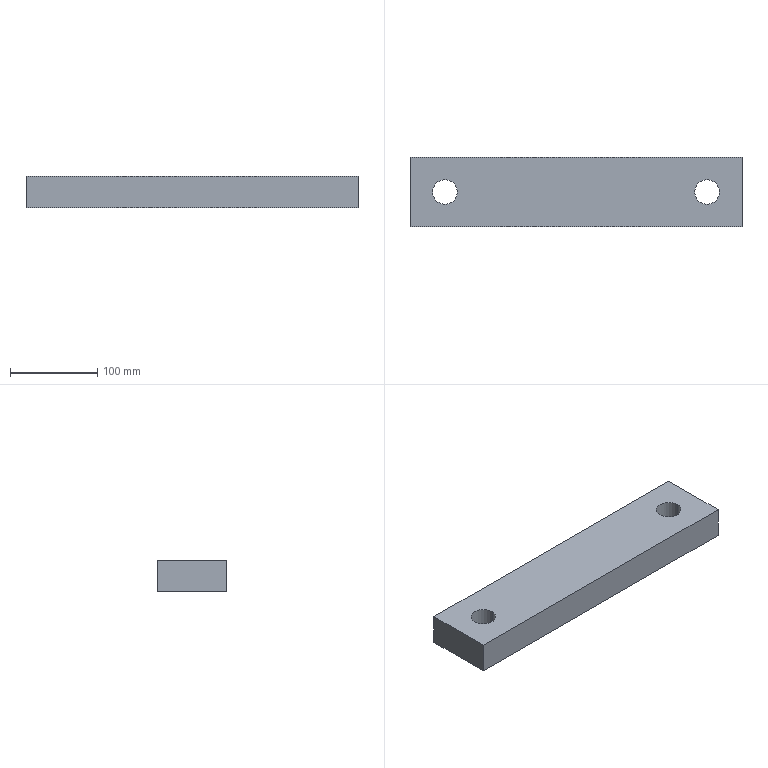Part | SolidWorks | features Extrusion 1, HoleWzd 1 | 1 solid | 10 faces | box 380 x 80 x 36 mm | volume 1049498 mm3 | plane 6 | cylinder 4 | commonest cylinder face diameters 28.179 x4
STEP:
#1=CARTESIAN_POINT('',(-164.089,0.,-18.));
#2=VERTEX_POINT('',#1);
#3=CARTESIAN_POINT('',(-135.911,0.,-18.));
#4=VERTEX_POINT('',#3);
#5=CARTESIAN_POINT('',(-150.,0.,-18.));
#6=DIRECTION('',(0.,0.,1.));
#7=DIRECTION('',(1.,0.,0.));
#8=AXIS2_PLACEMENT_3D('',#5,#6,#7);
#9=CIRCLE('',#8,14.089);
#10=EDGE_CURVE('',#2,#4,#9,.T.);
#11=ORIENTED_EDGE('',*,*,#10,.F.);
#12=CARTESIAN_POINT('',(-164.089,0.,18.));
#13=VERTEX_POINT('',#12);
#14=CARTESIAN_POINT('',(-164.089,0.,18.));
#15=DIRECTION('',(0.,0.,1.));
#16=VECTOR('',#15,1000.);
#17=LINE('',#14,#16);
#18=EDGE_CURVE('',#2,#13,#17,.T.);
#19=ORIENTED_EDGE('',*,*,#18,.T.);
#20=CARTESIAN_POINT('',(-135.911,0.,18.));
#21=VERTEX_POINT('',#20);
#22=CARTESIAN_POINT('',(-150.,0.,18.));
#23=DIRECTION('',(0.,0.,1.));
#24=DIRECTION('',(1.,0.,0.));
#25=AXIS2_PLACEMENT_3D('',#22,#23,#24);
#26=CIRCLE('',#25,14.089);
#27=EDGE_CURVE('',#13,#21,#26,.T.);
#28=ORIENTED_EDGE('',*,*,#27,.T.);
#29=CARTESIAN_POINT('',(-135.911,0.,18.));
#30=DIRECTION('',(0.,0.,1.));
#31=VECTOR('',#30,1000.);
#32=LINE('',#29,#31);
#33=EDGE_CURVE('',#4,#21,#32,.T.);
#34=ORIENTED_EDGE('',*,*,#33,.F.);
#35=EDGE_LOOP('',(#11,#19,#28,#34));
#36=FACE_OUTER_BOUND('',#35,.T.);
#37=CARTESIAN_POINT('',(-150.,0.,18.));
#38=DIRECTION('',(0.,0.,1.));
#39=DIRECTION('',(1.,0.,0.));
#40=AXIS2_PLACEMENT_3D('',#37,#38,#39);
#41=CYLINDRICAL_SURFACE('',#40,14.089);
#42=ADVANCED_FACE('',(#36),#41,.F.);
#43=CARTESIAN_POINT('',(135.911,0.,-18.));
#44=VERTEX_POINT('',#43);
#45=CARTESIAN_POINT('',(164.089,0.,-18.));
#46=VERTEX_POINT('',#45);
#47=CARTESIAN_POINT('',(150.,0.,-18.));
#48=DIRECTION('',(0.,0.,1.));
#49=DIRECTION('',(1.,0.,0.));
#50=AXIS2_PLACEMENT_3D('',#47,#48,#49);
#51=CIRCLE('',#50,14.089);
#52=EDGE_CURVE('',#44,#46,#51,.T.);
#53=ORIENTED_EDGE('',*,*,#52,.F.);
#54=CARTESIAN_POINT('',(135.911,0.,18.));
#55=VERTEX_POINT('',#54);
#56=CARTESIAN_POINT('',(135.911,0.,18.));
#57=DIRECTION('',(0.,0.,1.));
#58=VECTOR('',#57,1000.);
#59=LINE('',#56,#58);
#60=EDGE_CURVE('',#44,#55,#59,.T.);
#61=ORIENTED_EDGE('',*,*,#60,.T.);
#62=CARTESIAN_POINT('',(164.089,0.,18.));
#63=VERTEX_POINT('',#62);
#64=CARTESIAN_POINT('',(150.,0.,18.));
#65=DIRECTION('',(0.,0.,1.));
#66=DIRECTION('',(1.,0.,0.));
#67=AXIS2_PLACEMENT_3D('',#64,#65,#66);
#68=CIRCLE('',#67,14.089);
#69=EDGE_CURVE('',#55,#63,#68,.T.);
#70=ORIENTED_EDGE('',*,*,#69,.T.);
#71=CARTESIAN_POINT('',(164.089,0.,18.));
#72=DIRECTION('',(0.,0.,1.));
#73=VECTOR('',#72,1000.);
#74=LINE('',#71,#73);
#75=EDGE_CURVE('',#46,#63,#74,.T.);
#76=ORIENTED_EDGE('',*,*,#75,.F.);
#77=EDGE_LOOP('',(#53,#61,#70,#76));
#78=FACE_OUTER_BOUND('',#77,.T.);
#79=CARTESIAN_POINT('',(150.,0.,18.));
#80=DIRECTION('',(0.,0.,1.));
#81=DIRECTION('',(1.,0.,0.));
#82=AXIS2_PLACEMENT_3D('',#79,#80,#81);
#83=CYLINDRICAL_SURFACE('',#82,14.089);
#84=ADVANCED_FACE('',(#78),#83,.F.);
#85=CARTESIAN_POINT('',(-190.,40.,-18.));
#86=VERTEX_POINT('',#85);
#87=CARTESIAN_POINT('',(-190.,-40.,-18.));
#88=VERTEX_POINT('',#87);
#89=CARTESIAN_POINT('',(-190.,40.,-18.));
#90=DIRECTION('',(0.,-1.,0.));
#91=VECTOR('',#90,1000.);
#92=LINE('',#89,#91);
#93=EDGE_CURVE('',#86,#88,#92,.T.);
#94=ORIENTED_EDGE('',*,*,#93,.T.);
#95=CARTESIAN_POINT('',(-190.,-40.,18.));
#96=VERTEX_POINT('',#95);
#97=CARTESIAN_POINT('',(-190.,-40.,18.));
#98=DIRECTION('',(0.,0.,-1.));
#99=VECTOR('',#98,1000.);
#100=LINE('',#97,#99);
#101=EDGE_CURVE('',#96,#88,#100,.T.);
#102=ORIENTED_EDGE('',*,*,#101,.F.);
#103=CARTESIAN_POINT('',(-190.,40.,18.));
#104=VERTEX_POINT('',#103);
#105=CARTESIAN_POINT('',(-190.,40.,18.));
#106=DIRECTION('',(0.,-1.,0.));
#107=VECTOR('',#106,1000.);
#108=LINE('',#105,#107);
#109=EDGE_CURVE('',#104,#96,#108,.T.);
#110=ORIENTED_EDGE('',*,*,#109,.F.);
#111=CARTESIAN_POINT('',(-190.,40.,18.));
#112=DIRECTION('',(0.,0.,-1.));
#113=VECTOR('',#112,1000.);
#114=LINE('',#111,#113);
#115=EDGE_CURVE('',#104,#86,#114,.T.);
#116=ORIENTED_EDGE('',*,*,#115,.T.);
#117=EDGE_LOOP('',(#94,#102,#110,#116));
#118=FACE_OUTER_BOUND('',#117,.T.);
#119=CARTESIAN_POINT('',(-190.,40.,18.));
#120=DIRECTION('',(1.,0.,0.));
#121=DIRECTION('',(0.,1.,0.));
#122=AXIS2_PLACEMENT_3D('',#119,#120,#121);
#123=PLANE('',#122);
#124=ADVANCED_FACE('',(#118),#123,.F.);
#125=CARTESIAN_POINT('',(190.,-40.,-18.));
#126=VERTEX_POINT('',#125);
#127=CARTESIAN_POINT('',(-190.,-40.,-18.));
#128=DIRECTION('',(1.,0.,0.));
#129=VECTOR('',#128,1000.);
#130=LINE('',#127,#129);
#131=EDGE_CURVE('',#88,#126,#130,.T.);
#132=ORIENTED_EDGE('',*,*,#131,.T.);
#133=CARTESIAN_POINT('',(190.,-40.,18.));
#134=VERTEX_POINT('',#133);
#135=CARTESIAN_POINT('',(190.,-40.,18.));
#136=DIRECTION('',(0.,0.,-1.));
#137=VECTOR('',#136,1000.);
#138=LINE('',#135,#137);
#139=EDGE_CURVE('',#134,#126,#138,.T.);
#140=ORIENTED_EDGE('',*,*,#139,.F.);
#141=CARTESIAN_POINT('',(-190.,-40.,18.));
#142=DIRECTION('',(1.,0.,0.));
#143=VECTOR('',#142,1000.);
#144=LINE('',#141,#143);
#145=EDGE_CURVE('',#96,#134,#144,.T.);
#146=ORIENTED_EDGE('',*,*,#145,.F.);
#147=ORIENTED_EDGE('',*,*,#101,.T.);
#148=EDGE_LOOP('',(#132,#140,#146,#147));
#149=FACE_OUTER_BOUND('',#148,.T.);
#150=CARTESIAN_POINT('',(-190.,-40.,18.));
#151=DIRECTION('',(0.,1.,0.));
#152=DIRECTION('',(0.,0.,1.));
#153=AXIS2_PLACEMENT_3D('',#150,#151,#152);
#154=PLANE('',#153);
#155=ADVANCED_FACE('',(#149),#154,.F.);
#156=CARTESIAN_POINT('',(190.,40.,-18.));
#157=VERTEX_POINT('',#156);
#158=CARTESIAN_POINT('',(190.,40.,-18.));
#159=DIRECTION('',(0.,1.,0.));
#160=VECTOR('',#159,1000.);
#161=LINE('',#158,#160);
#162=EDGE_CURVE('',#126,#157,#161,.T.);
#163=ORIENTED_EDGE('',*,*,#162,.T.);
#164=CARTESIAN_POINT('',(190.,40.,18.));
#165=VERTEX_POINT('',#164);
#166=CARTESIAN_POINT('',(190.,40.,18.));
#167=DIRECTION('',(0.,0.,-1.));
#168=VECTOR('',#167,1000.);
#169=LINE('',#166,#168);
#170=EDGE_CURVE('',#165,#157,#169,.T.);
#171=ORIENTED_EDGE('',*,*,#170,.F.);
#172=CARTESIAN_POINT('',(190.,40.,18.));
#173=DIRECTION('',(0.,1.,0.));
#174=VECTOR('',#173,1000.);
#175=LINE('',#172,#174);
#176=EDGE_CURVE('',#134,#165,#175,.T.);
#177=ORIENTED_EDGE('',*,*,#176,.F.);
#178=ORIENTED_EDGE('',*,*,#139,.T.);
#179=EDGE_LOOP('',(#163,#171,#177,#178));
#180=FACE_OUTER_BOUND('',#179,.T.);
#181=CARTESIAN_POINT('',(190.,40.,18.));
#182=DIRECTION('',(-1.,0.,0.));
#183=DIRECTION('',(0.,0.,1.));
#184=AXIS2_PLACEMENT_3D('',#181,#182,#183);
#185=PLANE('',#184);
#186=ADVANCED_FACE('',(#180),#185,.F.);
#187=CARTESIAN_POINT('',(-190.,40.,-18.));
#188=DIRECTION('',(-1.,0.,0.));
#189=VECTOR('',#188,1000.);
#190=LINE('',#187,#189);
#191=EDGE_CURVE('',#157,#86,#190,.T.);
#192=ORIENTED_EDGE('',*,*,#191,.T.);
#193=ORIENTED_EDGE('',*,*,#115,.F.);
#194=CARTESIAN_POINT('',(-190.,40.,18.));
#195=DIRECTION('',(-1.,0.,0.));
#196=VECTOR('',#195,1000.);
#197=LINE('',#194,#196);
#198=EDGE_CURVE('',#165,#104,#197,.T.);
#199=ORIENTED_EDGE('',*,*,#198,.F.);
#200=ORIENTED_EDGE('',*,*,#170,.T.);
#201=EDGE_LOOP('',(#192,#193,#199,#200));
#202=FACE_OUTER_BOUND('',#201,.T.);
#203=CARTESIAN_POINT('',(-190.,40.,18.));
#204=DIRECTION('',(0.,-1.,0.));
#205=DIRECTION('',(1.,0.,0.));
#206=AXIS2_PLACEMENT_3D('',#203,#204,#205);
#207=PLANE('',#206);
#208=ADVANCED_FACE('',(#202),#207,.F.);
#209=CARTESIAN_POINT('',(-150.,0.,18.));
#210=DIRECTION('',(0.,0.,1.));
#211=DIRECTION('',(1.,0.,0.));
#212=AXIS2_PLACEMENT_3D('',#209,#210,#211);
#213=CIRCLE('',#212,14.089);
#214=EDGE_CURVE('',#21,#13,#213,.T.);
#215=ORIENTED_EDGE('',*,*,#214,.F.);
#216=ORIENTED_EDGE('',*,*,#27,.F.);
#217=EDGE_LOOP('',(#215,#216));
#218=FACE_BOUND('',#217,.T.);
#219=CARTESIAN_POINT('',(150.,0.,18.));
#220=DIRECTION('',(0.,0.,1.));
#221=DIRECTION('',(1.,0.,0.));
#222=AXIS2_PLACEMENT_3D('',#219,#220,#221);
#223=CIRCLE('',#222,14.089);
#224=EDGE_CURVE('',#63,#55,#223,.T.);
#225=ORIENTED_EDGE('',*,*,#224,.F.);
#226=ORIENTED_EDGE('',*,*,#69,.F.);
#227=EDGE_LOOP('',(#225,#226));
#228=FACE_BOUND('',#227,.T.);
#229=ORIENTED_EDGE('',*,*,#109,.T.);
#230=ORIENTED_EDGE('',*,*,#145,.T.);
#231=ORIENTED_EDGE('',*,*,#176,.T.);
#232=ORIENTED_EDGE('',*,*,#198,.T.);
#233=EDGE_LOOP('',(#229,#230,#231,#232));
#234=FACE_OUTER_BOUND('',#233,.T.);
#235=CARTESIAN_POINT('',(-190.,-40.,18.));
#236=DIRECTION('',(0.,0.,1.));
#237=DIRECTION('',(1.,0.,0.));
#238=AXIS2_PLACEMENT_3D('',#235,#236,#237);
#239=PLANE('',#238);
#240=ADVANCED_FACE('',(#218,#228,#234),#239,.T.);
#241=CARTESIAN_POINT('',(-150.,0.,-18.));
#242=DIRECTION('',(0.,0.,1.));
#243=DIRECTION('',(1.,0.,0.));
#244=AXIS2_PLACEMENT_3D('',#241,#242,#243);
#245=CIRCLE('',#244,14.089);
#246=EDGE_CURVE('',#4,#2,#245,.T.);
#247=ORIENTED_EDGE('',*,*,#246,.T.);
#248=ORIENTED_EDGE('',*,*,#10,.T.);
#249=EDGE_LOOP('',(#247,#248));
#250=FACE_BOUND('',#249,.T.);
#251=CARTESIAN_POINT('',(150.,0.,-18.));
#252=DIRECTION('',(0.,0.,1.));
#253=DIRECTION('',(1.,0.,0.));
#254=AXIS2_PLACEMENT_3D('',#251,#252,#253);
#255=CIRCLE('',#254,14.089);
#256=EDGE_CURVE('',#46,#44,#255,.T.);
#257=ORIENTED_EDGE('',*,*,#256,.T.);
#258=ORIENTED_EDGE('',*,*,#52,.T.);
#259=EDGE_LOOP('',(#257,#258));
#260=FACE_BOUND('',#259,.T.);
#261=ORIENTED_EDGE('',*,*,#93,.F.);
#262=ORIENTED_EDGE('',*,*,#191,.F.);
#263=ORIENTED_EDGE('',*,*,#162,.F.);
#264=ORIENTED_EDGE('',*,*,#131,.F.);
#265=EDGE_LOOP('',(#261,#262,#263,#264));
#266=FACE_OUTER_BOUND('',#265,.T.);
#267=CARTESIAN_POINT('',(-190.,-40.,-18.));
#268=DIRECTION('',(0.,0.,1.));
#269=DIRECTION('',(1.,0.,0.));
#270=AXIS2_PLACEMENT_3D('',#267,#268,#269);
#271=PLANE('',#270);
#272=ADVANCED_FACE('',(#250,#260,#266),#271,.F.);
#273=ORIENTED_EDGE('',*,*,#60,.F.);
#274=ORIENTED_EDGE('',*,*,#256,.F.);
#275=ORIENTED_EDGE('',*,*,#75,.T.);
#276=ORIENTED_EDGE('',*,*,#224,.T.);
#277=EDGE_LOOP('',(#273,#274,#275,#276));
#278=FACE_OUTER_BOUND('',#277,.T.);
#279=CARTESIAN_POINT('',(150.,0.,18.));
#280=DIRECTION('',(0.,0.,1.));
#281=DIRECTION('',(1.,0.,0.));
#282=AXIS2_PLACEMENT_3D('',#279,#280,#281);
#283=CYLINDRICAL_SURFACE('',#282,14.089);
#284=ADVANCED_FACE('',(#278),#283,.F.);
#285=ORIENTED_EDGE('',*,*,#18,.F.);
#286=ORIENTED_EDGE('',*,*,#246,.F.);
#287=ORIENTED_EDGE('',*,*,#33,.T.);
#288=ORIENTED_EDGE('',*,*,#214,.T.);
#289=EDGE_LOOP('',(#285,#286,#287,#288));
#290=FACE_OUTER_BOUND('',#289,.T.);
#291=CARTESIAN_POINT('',(-150.,0.,18.));
#292=DIRECTION('',(0.,0.,1.));
#293=DIRECTION('',(1.,0.,0.));
#294=AXIS2_PLACEMENT_3D('',#291,#292,#293);
#295=CYLINDRICAL_SURFACE('',#294,14.089);
#296=ADVANCED_FACE('',(#290),#295,.F.);
#297=CLOSED_SHELL('',(#42,#84,#124,#155,#186,#208,#240,#272,#284,#296));
#298=MANIFOLD_SOLID_BREP('',#297);
#299=CARTESIAN_POINT('',(0.,0.,0.));
#300=DIRECTION('',(0.,0.,1.));
#301=DIRECTION('',(1.,0.,0.));
#302=AXIS2_PLACEMENT_3D('',#299,#300,#301);
#303=(LENGTH_UNIT()NAMED_UNIT(*)SI_UNIT(.MILLI.,.METRE.));
#304=UNCERTAINTY_MEASURE_WITH_UNIT(LENGTH_MEASURE(0.00001),#303,'','');
#305=(NAMED_UNIT(*)PLANE_ANGLE_UNIT()SI_UNIT($,.RADIAN.));
#306=(NAMED_UNIT(*)SI_UNIT($,.STERADIAN.)SOLID_ANGLE_UNIT());
#307=(GEOMETRIC_REPRESENTATION_CONTEXT(3)GLOBAL_UNCERTAINTY_ASSIGNED_CONTEXT((#304))GLOBAL_UNIT_ASSIGNED_CONTEXT((#303,#305,#306))REPRESENTATION_CONTEXT('',''));
#308=ADVANCED_BREP_SHAPE_REPRESENTATION('',(#298,#302),#307);